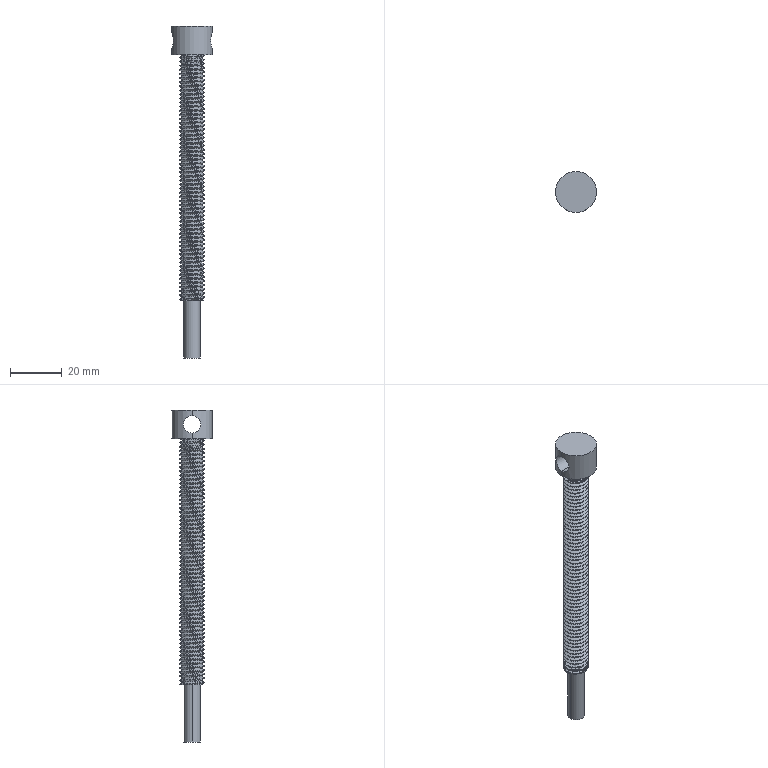Part | SolidWorks | features Helix 1, ICE 1, Revolution 1, SweepCut 1 | 1 solid | 134 faces | box 15.875 x 15.875 x 128.6 mm | volume 7890 mm3 | cylinder 127 | plane 4 | spline 3 | commonest cylinder face diameters 9.55 x121 6.35 x2 6.756 x2 15.875 x2